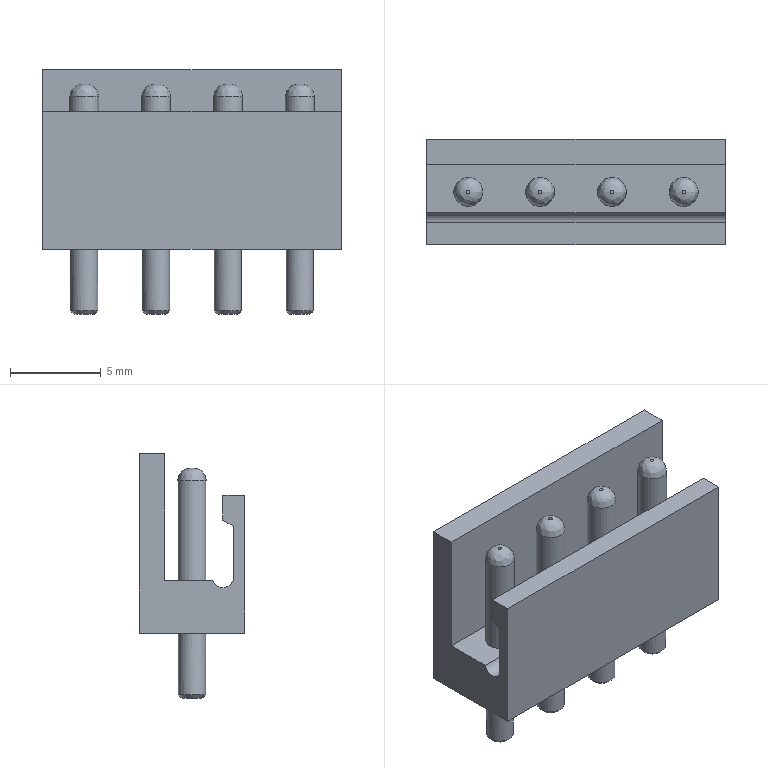Part | STEP file | JL27-04ZJB | 1 solid | 37 faces | box 16.44 x 5.8 x 13.5 mm | volume 568.163 mm3 | plane 20 | cylinder 9 | spline 4 | cone 4 | commonest cylinder face diameters 1.5 x4 1.59 x4 1.2 x1